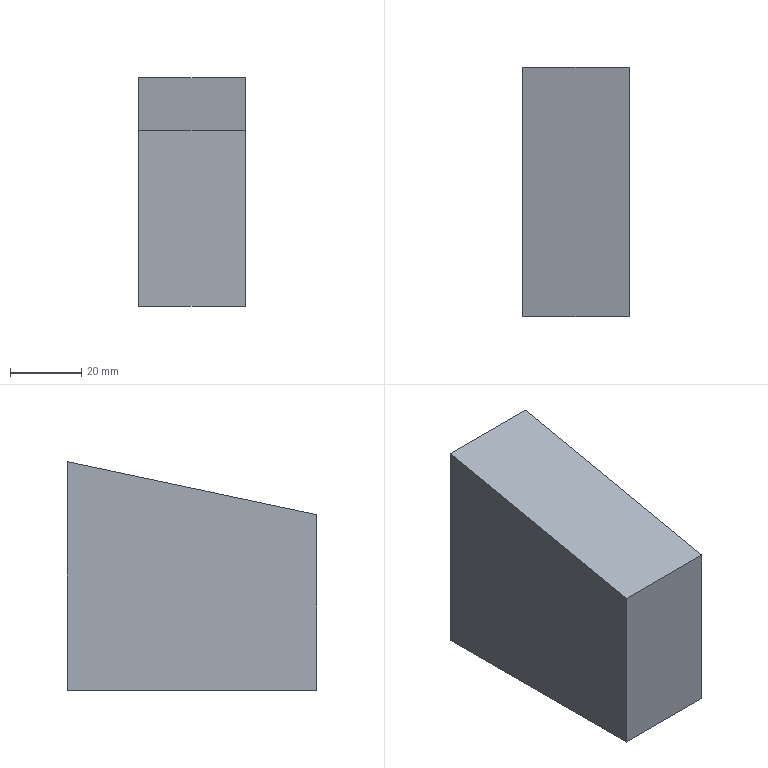Part | NX | features solid 2 | 1 solid | 6 faces | box 30 x 70 x 64.217 mm | volume 119233 mm3 | plane 6
STEP:
#1=CARTESIAN_POINT('',(380.,-640.,19.338));
#2=VERTEX_POINT('',#1);
#3=CARTESIAN_POINT('',(380.,-570.,34.217));
#4=VERTEX_POINT('',#3);
#5=CARTESIAN_POINT('',(380.,-620.323,23.521));
#6=DIRECTION('',(0.,0.9781,0.2079));
#7=VECTOR('',#6,1000.);
#8=LINE('',#5,#7);
#9=EDGE_CURVE('',#2,#4,#8,.T.);
#10=ORIENTED_EDGE('',*,*,#9,.T.);
#11=CARTESIAN_POINT('',(350.,-570.,34.217));
#12=VERTEX_POINT('',#11);
#13=CARTESIAN_POINT('',(380.,-570.,34.217));
#14=DIRECTION('',(-1.,0.,0.));
#15=VECTOR('',#14,1000.);
#16=LINE('',#13,#15);
#17=EDGE_CURVE('',#4,#12,#16,.T.);
#18=ORIENTED_EDGE('',*,*,#17,.T.);
#19=CARTESIAN_POINT('',(350.,-640.,19.338));
#20=VERTEX_POINT('',#19);
#21=CARTESIAN_POINT('',(350.,-620.323,23.521));
#22=DIRECTION('',(0.,0.9781,0.2079));
#23=VECTOR('',#22,1000.);
#24=LINE('',#21,#23);
#25=EDGE_CURVE('',#20,#12,#24,.T.);
#26=ORIENTED_EDGE('',*,*,#25,.F.);
#27=CARTESIAN_POINT('',(670.,-640.,19.338));
#28=DIRECTION('',(-1.,0.,0.));
#29=VECTOR('',#28,1000.);
#30=LINE('',#27,#29);
#31=EDGE_CURVE('',#2,#20,#30,.T.);
#32=ORIENTED_EDGE('',*,*,#31,.F.);
#33=EDGE_LOOP('',(#10,#18,#26,#32));
#34=FACE_BOUND('',#33,.T.);
#35=CARTESIAN_POINT('',(340.,-639.682,19.406));
#36=DIRECTION('',(0.,-0.2079,0.9781));
#37=DIRECTION('',(0.,-0.9781,-0.2079));
#38=AXIS2_PLACEMENT_3D('',#35,#36,#37);
#39=PLANE('',#38);
#40=ADVANCED_FACE('',(#34),#39,.T.);
#41=CARTESIAN_POINT('',(380.,-640.,-30.));
#42=VERTEX_POINT('',#41);
#43=CARTESIAN_POINT('',(380.,-640.,22.));
#44=DIRECTION('',(0.,0.,-1.));
#45=VECTOR('',#44,1000.);
#46=LINE('',#43,#45);
#47=EDGE_CURVE('',#2,#42,#46,.T.);
#48=ORIENTED_EDGE('',*,*,#47,.T.);
#49=CARTESIAN_POINT('',(380.,-570.,-30.));
#50=VERTEX_POINT('',#49);
#51=CARTESIAN_POINT('',(380.,-620.,-30.));
#52=DIRECTION('',(0.,1.,0.));
#53=VECTOR('',#52,1000.);
#54=LINE('',#51,#53);
#55=EDGE_CURVE('',#42,#50,#54,.T.);
#56=ORIENTED_EDGE('',*,*,#55,.T.);
#57=CARTESIAN_POINT('',(380.,-570.,22.));
#58=DIRECTION('',(0.,0.,-1.));
#59=VECTOR('',#58,1000.);
#60=LINE('',#57,#59);
#61=EDGE_CURVE('',#4,#50,#60,.T.);
#62=ORIENTED_EDGE('',*,*,#61,.F.);
#63=ORIENTED_EDGE('',*,*,#9,.F.);
#64=EDGE_LOOP('',(#48,#56,#62,#63));
#65=FACE_BOUND('',#64,.T.);
#66=CARTESIAN_POINT('',(380.,-620.,22.));
#67=DIRECTION('',(1.,0.,0.));
#68=DIRECTION('',(0.,0.,1.));
#69=AXIS2_PLACEMENT_3D('',#66,#67,#68);
#70=PLANE('',#69);
#71=ADVANCED_FACE('',(#65),#70,.T.);
#72=ORIENTED_EDGE('',*,*,#31,.T.);
#73=CARTESIAN_POINT('',(350.,-640.,-30.));
#74=VERTEX_POINT('',#73);
#75=CARTESIAN_POINT('',(350.,-640.,22.));
#76=DIRECTION('',(0.,0.,-1.));
#77=VECTOR('',#76,1000.);
#78=LINE('',#75,#77);
#79=EDGE_CURVE('',#20,#74,#78,.T.);
#80=ORIENTED_EDGE('',*,*,#79,.T.);
#81=CARTESIAN_POINT('',(670.,-640.,-30.));
#82=DIRECTION('',(-1.,0.,0.));
#83=VECTOR('',#82,1000.);
#84=LINE('',#81,#83);
#85=EDGE_CURVE('',#42,#74,#84,.T.);
#86=ORIENTED_EDGE('',*,*,#85,.F.);
#87=ORIENTED_EDGE('',*,*,#47,.F.);
#88=EDGE_LOOP('',(#72,#80,#86,#87));
#89=FACE_BOUND('',#88,.T.);
#90=CARTESIAN_POINT('',(670.,-640.,22.));
#91=DIRECTION('',(0.,1.,0.));
#92=DIRECTION('',(0.,0.,1.));
#93=AXIS2_PLACEMENT_3D('',#90,#91,#92);
#94=PLANE('',#93);
#95=ADVANCED_FACE('',(#89),#94,.F.);
#96=ORIENTED_EDGE('',*,*,#25,.T.);
#97=CARTESIAN_POINT('',(350.,-570.,-30.));
#98=VERTEX_POINT('',#97);
#99=CARTESIAN_POINT('',(350.,-570.,22.));
#100=DIRECTION('',(0.,0.,-1.));
#101=VECTOR('',#100,1000.);
#102=LINE('',#99,#101);
#103=EDGE_CURVE('',#12,#98,#102,.T.);
#104=ORIENTED_EDGE('',*,*,#103,.T.);
#105=CARTESIAN_POINT('',(350.,-620.,-30.));
#106=DIRECTION('',(0.,1.,0.));
#107=VECTOR('',#106,1000.);
#108=LINE('',#105,#107);
#109=EDGE_CURVE('',#74,#98,#108,.T.);
#110=ORIENTED_EDGE('',*,*,#109,.F.);
#111=ORIENTED_EDGE('',*,*,#79,.F.);
#112=EDGE_LOOP('',(#96,#104,#110,#111));
#113=FACE_BOUND('',#112,.T.);
#114=CARTESIAN_POINT('',(350.,-620.,22.));
#115=DIRECTION('',(1.,0.,0.));
#116=DIRECTION('',(0.,0.,1.));
#117=AXIS2_PLACEMENT_3D('',#114,#115,#116);
#118=PLANE('',#117);
#119=ADVANCED_FACE('',(#113),#118,.F.);
#120=ORIENTED_EDGE('',*,*,#61,.T.);
#121=CARTESIAN_POINT('',(380.,-570.,-30.));
#122=DIRECTION('',(-1.,0.,0.));
#123=VECTOR('',#122,1000.);
#124=LINE('',#121,#123);
#125=EDGE_CURVE('',#50,#98,#124,.T.);
#126=ORIENTED_EDGE('',*,*,#125,.T.);
#127=ORIENTED_EDGE('',*,*,#103,.F.);
#128=ORIENTED_EDGE('',*,*,#17,.F.);
#129=EDGE_LOOP('',(#120,#126,#127,#128));
#130=FACE_BOUND('',#129,.T.);
#131=CARTESIAN_POINT('',(380.,-570.,22.));
#132=DIRECTION('',(0.,1.,0.));
#133=DIRECTION('',(0.,0.,1.));
#134=AXIS2_PLACEMENT_3D('',#131,#132,#133);
#135=PLANE('',#134);
#136=ADVANCED_FACE('',(#130),#135,.T.);
#137=ORIENTED_EDGE('',*,*,#55,.F.);
#138=ORIENTED_EDGE('',*,*,#85,.T.);
#139=ORIENTED_EDGE('',*,*,#109,.T.);
#140=ORIENTED_EDGE('',*,*,#125,.F.);
#141=EDGE_LOOP('',(#137,#138,#139,#140));
#142=FACE_BOUND('',#141,.T.);
#143=CARTESIAN_POINT('',(445.,-540.,-30.));
#144=DIRECTION('',(0.,0.,1.));
#145=DIRECTION('',(-1.,0.,0.));
#146=AXIS2_PLACEMENT_3D('',#143,#144,#145);
#147=PLANE('',#146);
#148=ADVANCED_FACE('',(#142),#147,.F.);
#149=CLOSED_SHELL('',(#40,#71,#95,#119,#136,#148));
#150=MANIFOLD_SOLID_BREP('',#149);
#151=(LENGTH_UNIT()NAMED_UNIT(*)SI_UNIT(.MILLI.,.METRE.));
#152=UNCERTAINTY_MEASURE_WITH_UNIT(LENGTH_MEASURE(0.00001),#151,'','');
#153=(NAMED_UNIT(*)PLANE_ANGLE_UNIT()SI_UNIT($,.RADIAN.));
#154=(NAMED_UNIT(*)SI_UNIT($,.STERADIAN.)SOLID_ANGLE_UNIT());
#155=(GEOMETRIC_REPRESENTATION_CONTEXT(3)GLOBAL_UNCERTAINTY_ASSIGNED_CONTEXT((#152))GLOBAL_UNIT_ASSIGNED_CONTEXT((#151,#153,#154))REPRESENTATION_CONTEXT('',''));
#156=ADVANCED_BREP_SHAPE_REPRESENTATION('',(#150),#155);